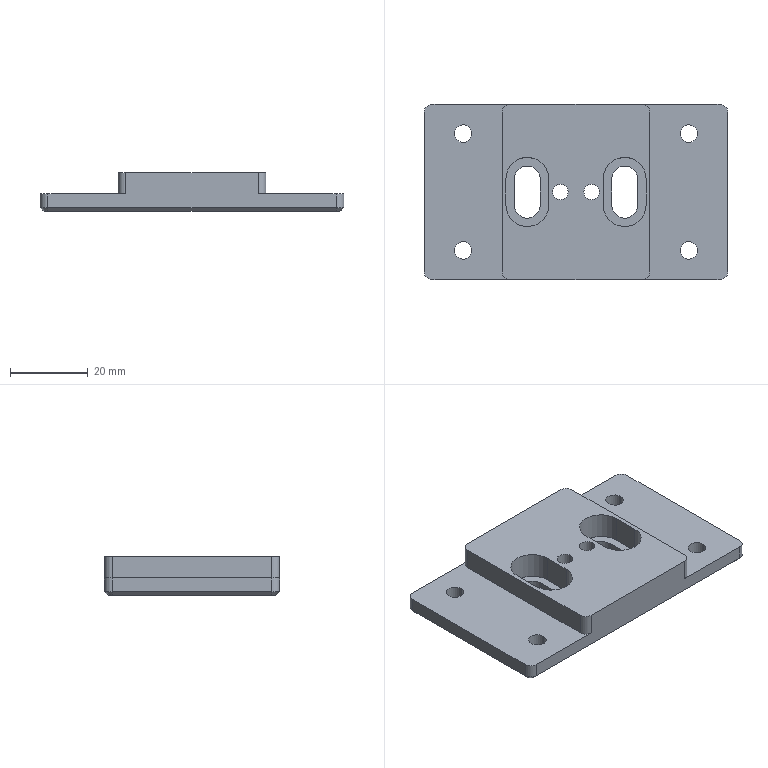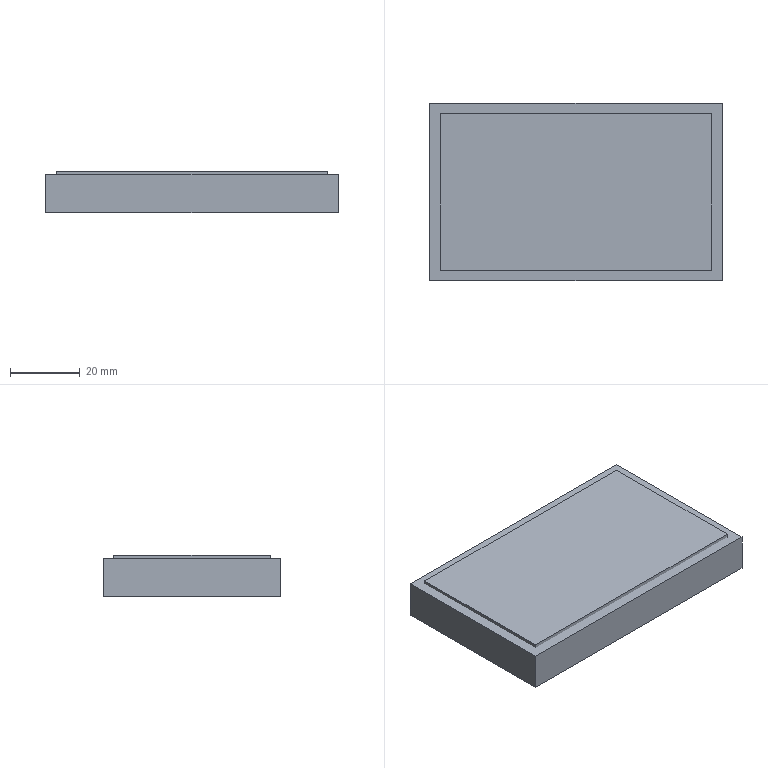CAM job | NX | 3-axis milling, drilling | part box 78 x 45 x 10 mm | stock box 84 x 51 x 12 mm
Tools:
number,name,description,diameter,corner_radius,flute_length,length,flutes
1,D63,Milling Tool-5 Parameters,63.0,0.0,50.0,75.0,2
10,D10,Milling Tool-5 Parameters,10.0,0.0,50.0,75.0,2
11,D10JING,Milling Tool-5 Parameters,10.0,0.0,50.0,75.0,2
6,D6,Milling Tool-5 Parameters,6.0,0.0,50.0,75.0,2
4,D4,Milling Tool-5 Parameters,4.0,0.0,50.0,75.0,2
7,D6A45,Milling Tool-5 Parameters,6.0,0.0,3.0,3.0,2
16,4.5ZT,Drilling Tool,4.5,0.0,35.0,50.0,2
13,3.8ZT,Drilling Tool,3.8,0.0,35.0,50.0,2
12,4.0JD,Milling Tool-5 Parameters,4.0,0.0,30.0,30.0,4
Operations:
program,operation,operation_type,tool,method,geometry_group,spindle_rpm,surface_speed,feed_per_tooth,feed_cut,feed_plunge,cut_length_mm,path_length_mm,cut_time_min,machine_time_min
1,FLOOR_WALL,VolumeBased25DMillingOperation,D63,METHOD,A,6500.0,1286.0,0.0962,1250.0,100.0,159.0,213.0,0.1272,0.1326
1,ADAPTIVE_MILLING,CavityMilling,D10,METHOD,A,9500.0,298.0,0.1579,3000.0,1000.0,6237.57,6543.313,2.081,2.112
1,ZLEVEL_PROFILE_COPY_COPY_1,ZLevelMilling,D10JING,METHOD,A,9500.0,298.0,0.0632,1200.0,100.0,282.022,356.022,0.235,0.2424
1,FLOOR_WALL_1,VolumeBased25DMillingOperation,D10JING,METHOD,A,9500.0,0.0,0.0,1250.0,100.0,609.938,1092.699,0.488,0.5362
1,ZLEVEL_PROFILE_COPY_COPY_1_COPY_1,ZLevelMilling,D6,METHOD,A,9500.0,179.0,0.1158,2200.0,100.0,933.897,1089.184,0.4245,0.44
1,ZLEVEL_PROFILE_COPY_COPY_1_COPY_2,ZLevelMilling,D6,METHOD,A,9500.0,298.0,0.0632,1200.0,100.0,74.354,234.72,0.062,0.078
1,ZLEVEL_PROFILE_COPY_COPY_1_COPY_1_COPY,ZLevelMilling,D4,METHOD,A,9500.0,119.0,0.0737,1400.0,100.0,581.929,757.49,0.4157,0.4332
1,DRILLING_COPY_1,Operation,D6A45,METHOD,A,5000.0,94.0,0.025,250.0,0.0,24.0,262.474,0.096,0.1198
1,DRILLING_COPY_COPY_1,Operation,4.5ZT,METHOD,A,2000.0,39.0,0.0375,150.0,0.0,41.408,281.192,0.2761,0.3
1,DRILLING_COPY_COPY_1_1,Operation,3.8ZT,METHOD,A,2000.0,39.0,0.0375,150.0,0.0,31.283,134.111,0.2086,0.2188
1,DRILLING_COPY_COPY_1_COPY,Operation,4.0JD,METHOD,A,1000.0,12.0,0.0125,50.0,0.0,27.0,125.544,0.54,0.5499
1,ZLEVEL_PROFILE_1_COPY_1_COPY,ZLevelMilling,D6A45,METHOD,A,9500.0,179.0,0.0526,1000.0,100.0,289.553,647.005,0.2896,0.3253
1,ZLEVEL_PROFILE_1_COPY_1_COPY_COPY,ZLevelMilling,D6A45,METHOD,A,9500.0,179.0,0.0526,1000.0,100.0,227.302,854.654,0.2273,0.29
2,FLOOR_WALL_COPY,VolumeBased25DMillingOperation,D63,METHOD,B,6500.0,1286.0,0.0962,1250.0,100.0,306.0,559,0.2448,0.2701
2,ZLEVEL_PROFILE_1_COPY_1_COPY_COPY_1,ZLevelMilling,D6A45,METHOD,B,9500.0,179.0,0.0526,1000.0,100.0,141.195,865.612,0.1412,0.2136
2,ZLEVEL_PROFILE_1_COPY_1_COPY_COPY_1_COPY,ZLevelMilling,D6A45,METHOD,B,9500.0,179.0,0.0526,1000.0,100.0,254.053,316.053,0.2541,0.2603